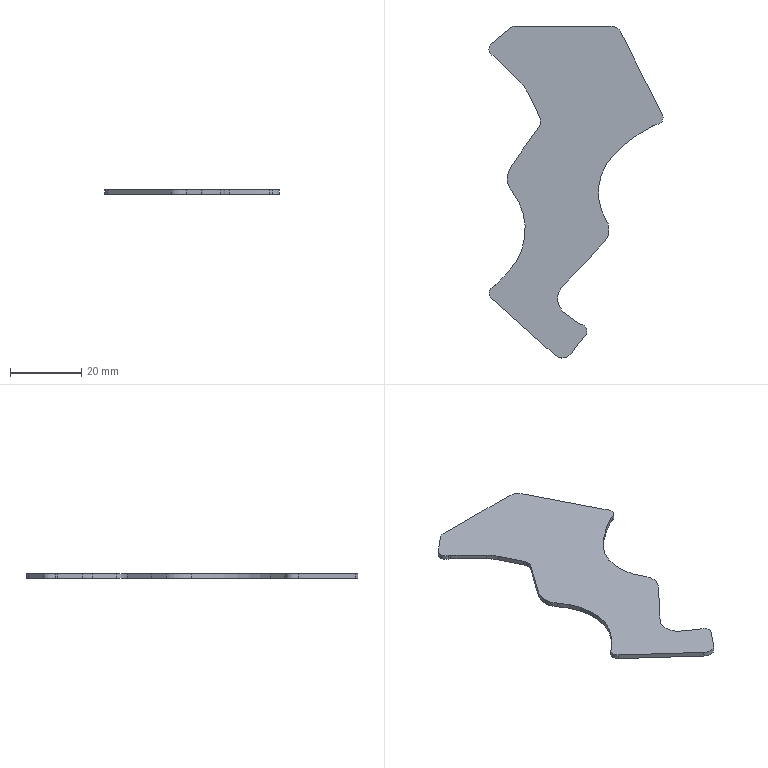Part | STEP file | gslz 2016.10.28-13_id154_x_t | 1 solid | 34 faces | box 48.815 x 93.009 x 1.25 mm | volume 2945 mm3 | cylinder 20 | plane 14 | commonest cylinder face diameters 4 x8 6 x4 10 x2 12 x1 20 x1 30 x1